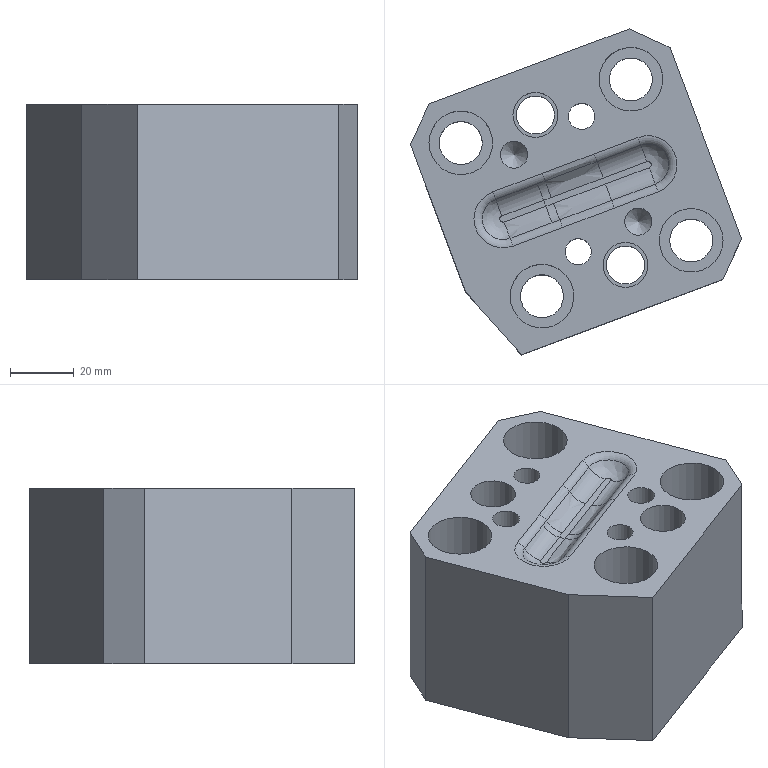Part | NX | features 23 2 | 1 solid | 58 faces | box 103.904 x 102.304 x 55 mm | volume 309293 mm3 | cylinder 26 | plane 20 | spline 8 | torus 2 | cone 2 | commonest cylinder face diameters 6 x4 13 x4 13.5 x4 20 x4 8.2 x2 8.5 x2